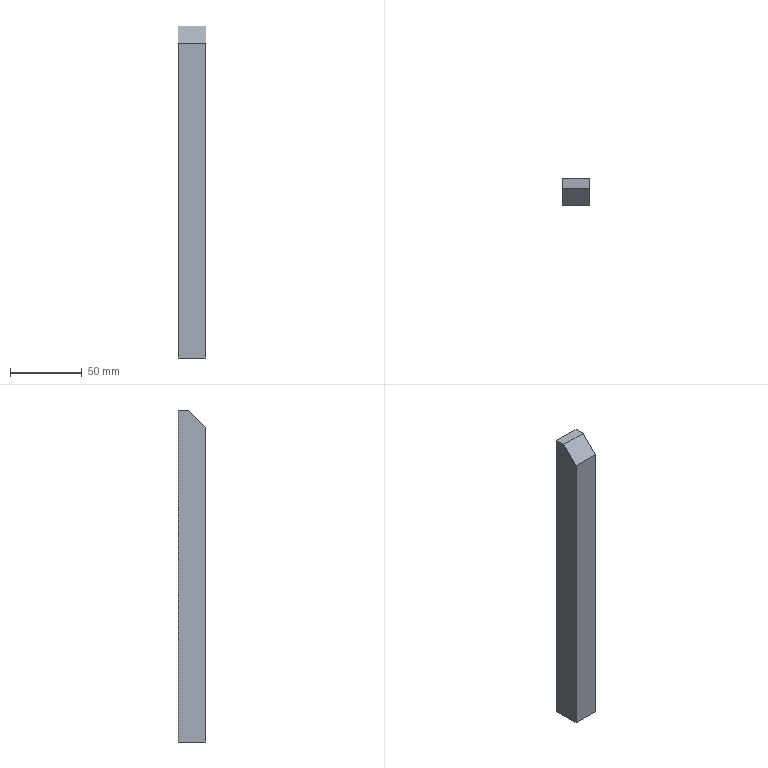Part | SolidWorks | features Chamfer 1, Extrusion 1 | 1 solid | 7 faces | box 19 x 19 x 231.5 mm | volume 82203 mm3 | plane 7
STEP:
#1=CARTESIAN_POINT('',(9.5,2.5,115.75));
#2=VERTEX_POINT('',#1);
#3=CARTESIAN_POINT('',(9.5,9.5,115.75));
#4=VERTEX_POINT('',#3);
#5=CARTESIAN_POINT('',(9.5,9.5,115.75));
#6=DIRECTION('',(0.,1.,0.));
#7=VECTOR('',#6,1000.);
#8=LINE('',#5,#7);
#9=EDGE_CURVE('',#2,#4,#8,.T.);
#10=ORIENTED_EDGE('',*,*,#9,.F.);
#11=CARTESIAN_POINT('',(9.5,-9.5,103.75));
#12=VERTEX_POINT('',#11);
#13=CARTESIAN_POINT('',(9.5,2.5,115.75));
#14=DIRECTION('',(0.,-0.7071,-0.7071));
#15=VECTOR('',#14,1000.);
#16=LINE('',#13,#15);
#17=EDGE_CURVE('',#2,#12,#16,.T.);
#18=ORIENTED_EDGE('',*,*,#17,.T.);
#19=CARTESIAN_POINT('',(9.5,-9.5,-115.75));
#20=VERTEX_POINT('',#19);
#21=CARTESIAN_POINT('',(9.5,-9.5,115.75));
#22=DIRECTION('',(0.,0.,-1.));
#23=VECTOR('',#22,1000.);
#24=LINE('',#21,#23);
#25=EDGE_CURVE('',#12,#20,#24,.T.);
#26=ORIENTED_EDGE('',*,*,#25,.T.);
#27=CARTESIAN_POINT('',(9.5,9.5,-115.75));
#28=VERTEX_POINT('',#27);
#29=CARTESIAN_POINT('',(9.5,9.5,-115.75));
#30=DIRECTION('',(0.,1.,0.));
#31=VECTOR('',#30,1000.);
#32=LINE('',#29,#31);
#33=EDGE_CURVE('',#20,#28,#32,.T.);
#34=ORIENTED_EDGE('',*,*,#33,.T.);
#35=CARTESIAN_POINT('',(9.5,9.5,115.75));
#36=DIRECTION('',(0.,0.,-1.));
#37=VECTOR('',#36,1000.);
#38=LINE('',#35,#37);
#39=EDGE_CURVE('',#4,#28,#38,.T.);
#40=ORIENTED_EDGE('',*,*,#39,.F.);
#41=EDGE_LOOP('',(#10,#18,#26,#34,#40));
#42=FACE_OUTER_BOUND('',#41,.T.);
#43=CARTESIAN_POINT('',(9.5,9.5,115.75));
#44=DIRECTION('',(-1.,0.,0.));
#45=DIRECTION('',(0.,-1.,0.));
#46=AXIS2_PLACEMENT_3D('',#43,#44,#45);
#47=PLANE('',#46);
#48=ADVANCED_FACE('',(#42),#47,.F.);
#49=CARTESIAN_POINT('',(-9.5,9.5,-115.75));
#50=VERTEX_POINT('',#49);
#51=CARTESIAN_POINT('',(-9.5,9.5,-115.75));
#52=DIRECTION('',(-1.,0.,0.));
#53=VECTOR('',#52,1000.);
#54=LINE('',#51,#53);
#55=EDGE_CURVE('',#28,#50,#54,.T.);
#56=ORIENTED_EDGE('',*,*,#55,.T.);
#57=CARTESIAN_POINT('',(-9.5,9.5,115.75));
#58=VERTEX_POINT('',#57);
#59=CARTESIAN_POINT('',(-9.5,9.5,115.75));
#60=DIRECTION('',(0.,0.,-1.));
#61=VECTOR('',#60,1000.);
#62=LINE('',#59,#61);
#63=EDGE_CURVE('',#58,#50,#62,.T.);
#64=ORIENTED_EDGE('',*,*,#63,.F.);
#65=CARTESIAN_POINT('',(-9.5,9.5,115.75));
#66=DIRECTION('',(-1.,0.,0.));
#67=VECTOR('',#66,1000.);
#68=LINE('',#65,#67);
#69=EDGE_CURVE('',#4,#58,#68,.T.);
#70=ORIENTED_EDGE('',*,*,#69,.F.);
#71=ORIENTED_EDGE('',*,*,#39,.T.);
#72=EDGE_LOOP('',(#56,#64,#70,#71));
#73=FACE_OUTER_BOUND('',#72,.T.);
#74=CARTESIAN_POINT('',(-9.5,9.5,115.75));
#75=DIRECTION('',(0.,-1.,0.));
#76=DIRECTION('',(0.,0.,-1.));
#77=AXIS2_PLACEMENT_3D('',#74,#75,#76);
#78=PLANE('',#77);
#79=ADVANCED_FACE('',(#73),#78,.F.);
#80=CARTESIAN_POINT('',(-9.5,-9.5,103.75));
#81=VERTEX_POINT('',#80);
#82=CARTESIAN_POINT('',(-9.5,-9.5,-115.75));
#83=VERTEX_POINT('',#82);
#84=CARTESIAN_POINT('',(-9.5,-9.5,115.75));
#85=DIRECTION('',(0.,0.,-1.));
#86=VECTOR('',#85,1000.);
#87=LINE('',#84,#86);
#88=EDGE_CURVE('',#81,#83,#87,.T.);
#89=ORIENTED_EDGE('',*,*,#88,.F.);
#90=CARTESIAN_POINT('',(-9.5,2.5,115.75));
#91=VERTEX_POINT('',#90);
#92=CARTESIAN_POINT('',(-9.5,2.5,115.75));
#93=DIRECTION('',(0.,0.7071,0.7071));
#94=VECTOR('',#93,1000.);
#95=LINE('',#92,#94);
#96=EDGE_CURVE('',#81,#91,#95,.T.);
#97=ORIENTED_EDGE('',*,*,#96,.T.);
#98=CARTESIAN_POINT('',(-9.5,9.5,115.75));
#99=DIRECTION('',(0.,-1.,0.));
#100=VECTOR('',#99,1000.);
#101=LINE('',#98,#100);
#102=EDGE_CURVE('',#58,#91,#101,.T.);
#103=ORIENTED_EDGE('',*,*,#102,.F.);
#104=ORIENTED_EDGE('',*,*,#63,.T.);
#105=CARTESIAN_POINT('',(-9.5,9.5,-115.75));
#106=DIRECTION('',(0.,-1.,0.));
#107=VECTOR('',#106,1000.);
#108=LINE('',#105,#107);
#109=EDGE_CURVE('',#50,#83,#108,.T.);
#110=ORIENTED_EDGE('',*,*,#109,.T.);
#111=EDGE_LOOP('',(#89,#97,#103,#104,#110));
#112=FACE_OUTER_BOUND('',#111,.T.);
#113=CARTESIAN_POINT('',(-9.5,9.5,115.75));
#114=DIRECTION('',(1.,0.,0.));
#115=DIRECTION('',(0.,0.,-1.));
#116=AXIS2_PLACEMENT_3D('',#113,#114,#115);
#117=PLANE('',#116);
#118=ADVANCED_FACE('',(#112),#117,.F.);
#119=ORIENTED_EDGE('',*,*,#25,.F.);
#120=CARTESIAN_POINT('',(-9.5,-9.5,103.75));
#121=DIRECTION('',(-1.,0.,0.));
#122=VECTOR('',#121,1000.);
#123=LINE('',#120,#122);
#124=EDGE_CURVE('',#12,#81,#123,.T.);
#125=ORIENTED_EDGE('',*,*,#124,.T.);
#126=ORIENTED_EDGE('',*,*,#88,.T.);
#127=CARTESIAN_POINT('',(-9.5,-9.5,-115.75));
#128=DIRECTION('',(1.,0.,0.));
#129=VECTOR('',#128,1000.);
#130=LINE('',#127,#129);
#131=EDGE_CURVE('',#83,#20,#130,.T.);
#132=ORIENTED_EDGE('',*,*,#131,.T.);
#133=EDGE_LOOP('',(#119,#125,#126,#132));
#134=FACE_OUTER_BOUND('',#133,.T.);
#135=CARTESIAN_POINT('',(-9.5,-9.5,115.75));
#136=DIRECTION('',(0.,1.,0.));
#137=DIRECTION('',(0.,0.,1.));
#138=AXIS2_PLACEMENT_3D('',#135,#136,#137);
#139=PLANE('',#138);
#140=ADVANCED_FACE('',(#134),#139,.F.);
#141=ORIENTED_EDGE('',*,*,#102,.T.);
#142=CARTESIAN_POINT('',(9.5,2.5,115.75));
#143=DIRECTION('',(1.,0.,0.));
#144=VECTOR('',#143,1000.);
#145=LINE('',#142,#144);
#146=EDGE_CURVE('',#91,#2,#145,.T.);
#147=ORIENTED_EDGE('',*,*,#146,.T.);
#148=ORIENTED_EDGE('',*,*,#9,.T.);
#149=ORIENTED_EDGE('',*,*,#69,.T.);
#150=EDGE_LOOP('',(#141,#147,#148,#149));
#151=FACE_OUTER_BOUND('',#150,.T.);
#152=CARTESIAN_POINT('',(0.,0.,115.75));
#153=DIRECTION('',(0.,0.,1.));
#154=DIRECTION('',(1.,0.,0.));
#155=AXIS2_PLACEMENT_3D('',#152,#153,#154);
#156=PLANE('',#155);
#157=ADVANCED_FACE('',(#151),#156,.T.);
#158=ORIENTED_EDGE('',*,*,#33,.F.);
#159=ORIENTED_EDGE('',*,*,#131,.F.);
#160=ORIENTED_EDGE('',*,*,#109,.F.);
#161=ORIENTED_EDGE('',*,*,#55,.F.);
#162=EDGE_LOOP('',(#158,#159,#160,#161));
#163=FACE_OUTER_BOUND('',#162,.T.);
#164=CARTESIAN_POINT('',(0.,0.,-115.75));
#165=DIRECTION('',(0.,0.,1.));
#166=DIRECTION('',(1.,0.,0.));
#167=AXIS2_PLACEMENT_3D('',#164,#165,#166);
#168=PLANE('',#167);
#169=ADVANCED_FACE('',(#163),#168,.F.);
#170=ORIENTED_EDGE('',*,*,#96,.F.);
#171=ORIENTED_EDGE('',*,*,#124,.F.);
#172=ORIENTED_EDGE('',*,*,#17,.F.);
#173=ORIENTED_EDGE('',*,*,#146,.F.);
#174=EDGE_LOOP('',(#170,#171,#172,#173));
#175=FACE_OUTER_BOUND('',#174,.T.);
#176=CARTESIAN_POINT('',(0.,2.5,115.75));
#177=DIRECTION('',(0.,-0.7071,0.7071));
#178=DIRECTION('',(-1.,0.,0.));
#179=AXIS2_PLACEMENT_3D('',#176,#177,#178);
#180=PLANE('',#179);
#181=ADVANCED_FACE('',(#175),#180,.T.);
#182=CLOSED_SHELL('',(#48,#79,#118,#140,#157,#169,#181));
#183=MANIFOLD_SOLID_BREP('',#182);
#184=CARTESIAN_POINT('',(0.,0.,0.));
#185=DIRECTION('',(0.,0.,1.));
#186=DIRECTION('',(1.,0.,0.));
#187=AXIS2_PLACEMENT_3D('',#184,#185,#186);
#188=(LENGTH_UNIT()NAMED_UNIT(*)SI_UNIT(.MILLI.,.METRE.));
#189=UNCERTAINTY_MEASURE_WITH_UNIT(LENGTH_MEASURE(0.00001),#188,'','');
#190=(NAMED_UNIT(*)PLANE_ANGLE_UNIT()SI_UNIT($,.RADIAN.));
#191=(NAMED_UNIT(*)SI_UNIT($,.STERADIAN.)SOLID_ANGLE_UNIT());
#192=(GEOMETRIC_REPRESENTATION_CONTEXT(3)GLOBAL_UNCERTAINTY_ASSIGNED_CONTEXT((#189))GLOBAL_UNIT_ASSIGNED_CONTEXT((#188,#190,#191))REPRESENTATION_CONTEXT('',''));
#193=ADVANCED_BREP_SHAPE_REPRESENTATION('',(#183,#187),#192);